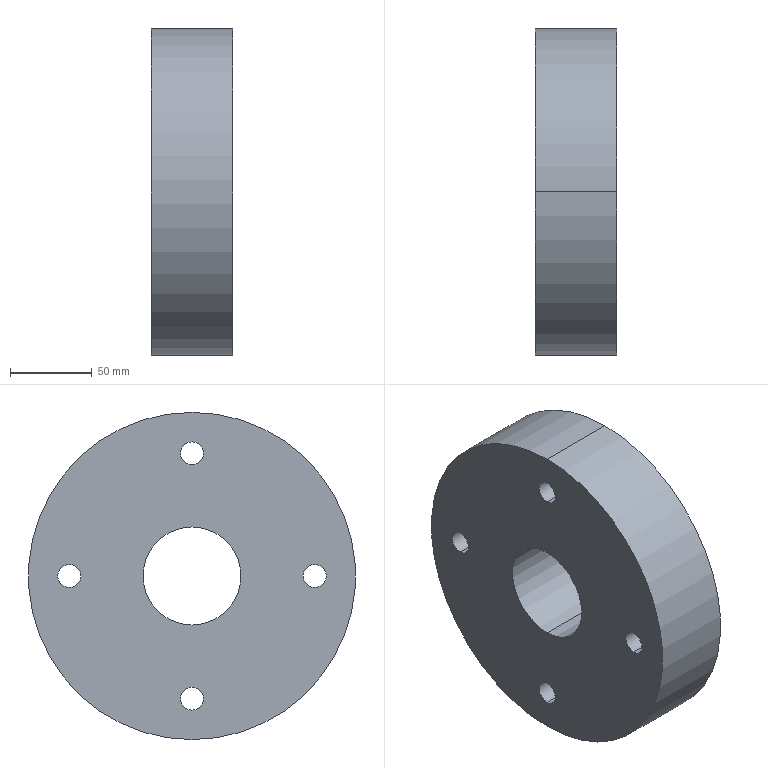Part | SolidWorks | features 3DProfileFeature 1, CirPattern 1, HoleWzd 1, Revolution 1 | 1 solid | 14 faces | box 50 x 200 x 200 mm | volume 1398637 mm3 | cylinder 12 | plane 2 | commonest cylinder face diameters 14 x8 60 x2 200 x2
STEP:
#1=CARTESIAN_POINT('',(25.,-75.,-7.));
#2=VERTEX_POINT('',#1);
#3=CARTESIAN_POINT('',(25.,-75.,7.));
#4=VERTEX_POINT('',#3);
#5=CARTESIAN_POINT('',(25.,-75.,0.));
#6=DIRECTION('',(-1.,0.,0.));
#7=DIRECTION('',(0.,0.,1.));
#8=AXIS2_PLACEMENT_3D('',#5,#6,#7);
#9=CIRCLE('',#8,7.);
#10=EDGE_CURVE('',#2,#4,#9,.T.);
#11=ORIENTED_EDGE('',*,*,#10,.F.);
#12=CARTESIAN_POINT('',(-25.,-75.,-7.));
#13=VERTEX_POINT('',#12);
#14=CARTESIAN_POINT('',(-25.,-75.,-7.));
#15=DIRECTION('',(-1.,0.,0.));
#16=VECTOR('',#15,1000.);
#17=LINE('',#14,#16);
#18=EDGE_CURVE('',#2,#13,#17,.T.);
#19=ORIENTED_EDGE('',*,*,#18,.T.);
#20=CARTESIAN_POINT('',(-25.,-75.,7.));
#21=VERTEX_POINT('',#20);
#22=CARTESIAN_POINT('',(-25.,-75.,0.));
#23=DIRECTION('',(-1.,0.,0.));
#24=DIRECTION('',(0.,0.,1.));
#25=AXIS2_PLACEMENT_3D('',#22,#23,#24);
#26=CIRCLE('',#25,7.);
#27=EDGE_CURVE('',#13,#21,#26,.T.);
#28=ORIENTED_EDGE('',*,*,#27,.T.);
#29=CARTESIAN_POINT('',(-25.,-75.,7.));
#30=DIRECTION('',(-1.,0.,0.));
#31=VECTOR('',#30,1000.);
#32=LINE('',#29,#31);
#33=EDGE_CURVE('',#4,#21,#32,.T.);
#34=ORIENTED_EDGE('',*,*,#33,.F.);
#35=EDGE_LOOP('',(#11,#19,#28,#34));
#36=FACE_OUTER_BOUND('',#35,.T.);
#37=CARTESIAN_POINT('',(-25.,-75.,0.));
#38=DIRECTION('',(-1.,0.,0.));
#39=DIRECTION('',(0.,0.,1.));
#40=AXIS2_PLACEMENT_3D('',#37,#38,#39);
#41=CYLINDRICAL_SURFACE('',#40,7.);
#42=ADVANCED_FACE('',(#36),#41,.F.);
#43=CARTESIAN_POINT('',(25.,0.,68.));
#44=VERTEX_POINT('',#43);
#45=CARTESIAN_POINT('',(25.,0.,82.));
#46=VERTEX_POINT('',#45);
#47=CARTESIAN_POINT('',(25.,0.,75.));
#48=DIRECTION('',(-1.,0.,0.));
#49=DIRECTION('',(0.,0.,1.));
#50=AXIS2_PLACEMENT_3D('',#47,#48,#49);
#51=CIRCLE('',#50,7.);
#52=EDGE_CURVE('',#44,#46,#51,.T.);
#53=ORIENTED_EDGE('',*,*,#52,.F.);
#54=CARTESIAN_POINT('',(-25.,0.,68.));
#55=VERTEX_POINT('',#54);
#56=CARTESIAN_POINT('',(-25.,0.,68.));
#57=DIRECTION('',(-1.,0.,0.));
#58=VECTOR('',#57,1000.);
#59=LINE('',#56,#58);
#60=EDGE_CURVE('',#44,#55,#59,.T.);
#61=ORIENTED_EDGE('',*,*,#60,.T.);
#62=CARTESIAN_POINT('',(-25.,0.,82.));
#63=VERTEX_POINT('',#62);
#64=CARTESIAN_POINT('',(-25.,0.,75.));
#65=DIRECTION('',(-1.,0.,0.));
#66=DIRECTION('',(0.,0.,1.));
#67=AXIS2_PLACEMENT_3D('',#64,#65,#66);
#68=CIRCLE('',#67,7.);
#69=EDGE_CURVE('',#55,#63,#68,.T.);
#70=ORIENTED_EDGE('',*,*,#69,.T.);
#71=CARTESIAN_POINT('',(-25.,0.,82.));
#72=DIRECTION('',(-1.,0.,0.));
#73=VECTOR('',#72,1000.);
#74=LINE('',#71,#73);
#75=EDGE_CURVE('',#46,#63,#74,.T.);
#76=ORIENTED_EDGE('',*,*,#75,.F.);
#77=EDGE_LOOP('',(#53,#61,#70,#76));
#78=FACE_OUTER_BOUND('',#77,.T.);
#79=CARTESIAN_POINT('',(-25.,0.,75.));
#80=DIRECTION('',(-1.,0.,0.));
#81=DIRECTION('',(0.,0.,1.));
#82=AXIS2_PLACEMENT_3D('',#79,#80,#81);
#83=CYLINDRICAL_SURFACE('',#82,7.);
#84=ADVANCED_FACE('',(#78),#83,.F.);
#85=CARTESIAN_POINT('',(25.,75.,-7.));
#86=VERTEX_POINT('',#85);
#87=CARTESIAN_POINT('',(25.,75.,7.));
#88=VERTEX_POINT('',#87);
#89=CARTESIAN_POINT('',(25.,75.,0.));
#90=DIRECTION('',(-1.,0.,0.));
#91=DIRECTION('',(0.,0.,1.));
#92=AXIS2_PLACEMENT_3D('',#89,#90,#91);
#93=CIRCLE('',#92,7.);
#94=EDGE_CURVE('',#86,#88,#93,.T.);
#95=ORIENTED_EDGE('',*,*,#94,.F.);
#96=CARTESIAN_POINT('',(-25.,75.,-7.));
#97=VERTEX_POINT('',#96);
#98=CARTESIAN_POINT('',(-25.,75.,-7.));
#99=DIRECTION('',(-1.,0.,0.));
#100=VECTOR('',#99,1000.);
#101=LINE('',#98,#100);
#102=EDGE_CURVE('',#86,#97,#101,.T.);
#103=ORIENTED_EDGE('',*,*,#102,.T.);
#104=CARTESIAN_POINT('',(-25.,75.,7.));
#105=VERTEX_POINT('',#104);
#106=CARTESIAN_POINT('',(-25.,75.,0.));
#107=DIRECTION('',(-1.,0.,0.));
#108=DIRECTION('',(0.,0.,1.));
#109=AXIS2_PLACEMENT_3D('',#106,#107,#108);
#110=CIRCLE('',#109,7.);
#111=EDGE_CURVE('',#97,#105,#110,.T.);
#112=ORIENTED_EDGE('',*,*,#111,.T.);
#113=CARTESIAN_POINT('',(-25.,75.,7.));
#114=DIRECTION('',(-1.,0.,0.));
#115=VECTOR('',#114,1000.);
#116=LINE('',#113,#115);
#117=EDGE_CURVE('',#88,#105,#116,.T.);
#118=ORIENTED_EDGE('',*,*,#117,.F.);
#119=EDGE_LOOP('',(#95,#103,#112,#118));
#120=FACE_OUTER_BOUND('',#119,.T.);
#121=CARTESIAN_POINT('',(-25.,75.,0.));
#122=DIRECTION('',(-1.,0.,0.));
#123=DIRECTION('',(0.,0.,1.));
#124=AXIS2_PLACEMENT_3D('',#121,#122,#123);
#125=CYLINDRICAL_SURFACE('',#124,7.);
#126=ADVANCED_FACE('',(#120),#125,.F.);
#127=CARTESIAN_POINT('',(25.,0.,-82.));
#128=VERTEX_POINT('',#127);
#129=CARTESIAN_POINT('',(25.,0.,-68.));
#130=VERTEX_POINT('',#129);
#131=CARTESIAN_POINT('',(25.,0.,-75.));
#132=DIRECTION('',(-1.,0.,0.));
#133=DIRECTION('',(0.,0.,1.));
#134=AXIS2_PLACEMENT_3D('',#131,#132,#133);
#135=CIRCLE('',#134,7.);
#136=EDGE_CURVE('',#128,#130,#135,.T.);
#137=ORIENTED_EDGE('',*,*,#136,.F.);
#138=CARTESIAN_POINT('',(-25.,0.,-82.));
#139=VERTEX_POINT('',#138);
#140=CARTESIAN_POINT('',(-25.,0.,-82.));
#141=DIRECTION('',(-1.,0.,0.));
#142=VECTOR('',#141,1000.);
#143=LINE('',#140,#142);
#144=EDGE_CURVE('',#128,#139,#143,.T.);
#145=ORIENTED_EDGE('',*,*,#144,.T.);
#146=CARTESIAN_POINT('',(-25.,0.,-68.));
#147=VERTEX_POINT('',#146);
#148=CARTESIAN_POINT('',(-25.,0.,-75.));
#149=DIRECTION('',(-1.,0.,0.));
#150=DIRECTION('',(0.,0.,1.));
#151=AXIS2_PLACEMENT_3D('',#148,#149,#150);
#152=CIRCLE('',#151,7.);
#153=EDGE_CURVE('',#139,#147,#152,.T.);
#154=ORIENTED_EDGE('',*,*,#153,.T.);
#155=CARTESIAN_POINT('',(-25.,0.,-68.));
#156=DIRECTION('',(-1.,0.,0.));
#157=VECTOR('',#156,1000.);
#158=LINE('',#155,#157);
#159=EDGE_CURVE('',#130,#147,#158,.T.);
#160=ORIENTED_EDGE('',*,*,#159,.F.);
#161=EDGE_LOOP('',(#137,#145,#154,#160));
#162=FACE_OUTER_BOUND('',#161,.T.);
#163=CARTESIAN_POINT('',(-25.,0.,-75.));
#164=DIRECTION('',(-1.,0.,0.));
#165=DIRECTION('',(0.,0.,1.));
#166=AXIS2_PLACEMENT_3D('',#163,#164,#165);
#167=CYLINDRICAL_SURFACE('',#166,7.);
#168=ADVANCED_FACE('',(#162),#167,.F.);
#169=CARTESIAN_POINT('',(-25.,0.,-100.));
#170=VERTEX_POINT('',#169);
#171=CARTESIAN_POINT('',(-25.,0.,100.));
#172=VERTEX_POINT('',#171);
#173=CARTESIAN_POINT('',(-25.,0.,0.));
#174=DIRECTION('',(1.,0.,0.));
#175=DIRECTION('',(0.,0.,-1.));
#176=AXIS2_PLACEMENT_3D('',#173,#174,#175);
#177=CIRCLE('',#176,100.);
#178=EDGE_CURVE('',#170,#172,#177,.T.);
#179=ORIENTED_EDGE('',*,*,#178,.T.);
#180=CARTESIAN_POINT('',(25.,0.,100.));
#181=VERTEX_POINT('',#180);
#182=CARTESIAN_POINT('',(71.901,0.,100.));
#183=DIRECTION('',(1.,0.,0.));
#184=VECTOR('',#183,1000.);
#185=LINE('',#182,#184);
#186=EDGE_CURVE('',#172,#181,#185,.T.);
#187=ORIENTED_EDGE('',*,*,#186,.T.);
#188=CARTESIAN_POINT('',(25.,0.,-100.));
#189=VERTEX_POINT('',#188);
#190=CARTESIAN_POINT('',(25.,0.,0.));
#191=DIRECTION('',(1.,0.,0.));
#192=DIRECTION('',(0.,0.,-1.));
#193=AXIS2_PLACEMENT_3D('',#190,#191,#192);
#194=CIRCLE('',#193,100.);
#195=EDGE_CURVE('',#189,#181,#194,.T.);
#196=ORIENTED_EDGE('',*,*,#195,.F.);
#197=CARTESIAN_POINT('',(71.901,0.,-100.));
#198=DIRECTION('',(1.,0.,0.));
#199=VECTOR('',#198,1000.);
#200=LINE('',#197,#199);
#201=EDGE_CURVE('',#170,#189,#200,.T.);
#202=ORIENTED_EDGE('',*,*,#201,.F.);
#203=EDGE_LOOP('',(#179,#187,#196,#202));
#204=FACE_OUTER_BOUND('',#203,.T.);
#205=CARTESIAN_POINT('',(71.901,0.,0.));
#206=DIRECTION('',(1.,0.,0.));
#207=DIRECTION('',(0.,0.,-1.));
#208=AXIS2_PLACEMENT_3D('',#205,#206,#207);
#209=CYLINDRICAL_SURFACE('',#208,100.);
#210=ADVANCED_FACE('',(#204),#209,.T.);
#211=CARTESIAN_POINT('',(-25.,0.,30.));
#212=VERTEX_POINT('',#211);
#213=CARTESIAN_POINT('',(-25.,0.,-30.));
#214=VERTEX_POINT('',#213);
#215=CARTESIAN_POINT('',(-25.,0.,0.));
#216=DIRECTION('',(1.,0.,0.));
#217=DIRECTION('',(0.,0.,-1.));
#218=AXIS2_PLACEMENT_3D('',#215,#216,#217);
#219=CIRCLE('',#218,30.);
#220=EDGE_CURVE('',#212,#214,#219,.T.);
#221=ORIENTED_EDGE('',*,*,#220,.F.);
#222=CARTESIAN_POINT('',(25.,0.,30.));
#223=VERTEX_POINT('',#222);
#224=CARTESIAN_POINT('',(71.901,0.,30.));
#225=DIRECTION('',(1.,0.,0.));
#226=VECTOR('',#225,1000.);
#227=LINE('',#224,#226);
#228=EDGE_CURVE('',#212,#223,#227,.T.);
#229=ORIENTED_EDGE('',*,*,#228,.T.);
#230=CARTESIAN_POINT('',(25.,0.,-30.));
#231=VERTEX_POINT('',#230);
#232=CARTESIAN_POINT('',(25.,0.,0.));
#233=DIRECTION('',(1.,0.,0.));
#234=DIRECTION('',(0.,0.,-1.));
#235=AXIS2_PLACEMENT_3D('',#232,#233,#234);
#236=CIRCLE('',#235,30.);
#237=EDGE_CURVE('',#223,#231,#236,.T.);
#238=ORIENTED_EDGE('',*,*,#237,.T.);
#239=CARTESIAN_POINT('',(71.901,0.,-30.));
#240=DIRECTION('',(1.,0.,0.));
#241=VECTOR('',#240,1000.);
#242=LINE('',#239,#241);
#243=EDGE_CURVE('',#214,#231,#242,.T.);
#244=ORIENTED_EDGE('',*,*,#243,.F.);
#245=EDGE_LOOP('',(#221,#229,#238,#244));
#246=FACE_OUTER_BOUND('',#245,.T.);
#247=CARTESIAN_POINT('',(71.901,0.,0.));
#248=DIRECTION('',(1.,0.,0.));
#249=DIRECTION('',(0.,0.,-1.));
#250=AXIS2_PLACEMENT_3D('',#247,#248,#249);
#251=CYLINDRICAL_SURFACE('',#250,30.);
#252=ADVANCED_FACE('',(#246),#251,.F.);
#253=CARTESIAN_POINT('',(25.,-75.,0.));
#254=DIRECTION('',(-1.,0.,0.));
#255=DIRECTION('',(0.,0.,1.));
#256=AXIS2_PLACEMENT_3D('',#253,#254,#255);
#257=CIRCLE('',#256,7.);
#258=EDGE_CURVE('',#4,#2,#257,.T.);
#259=ORIENTED_EDGE('',*,*,#258,.T.);
#260=ORIENTED_EDGE('',*,*,#10,.T.);
#261=EDGE_LOOP('',(#259,#260));
#262=FACE_BOUND('',#261,.T.);
#263=CARTESIAN_POINT('',(25.,0.,75.));
#264=DIRECTION('',(-1.,0.,0.));
#265=DIRECTION('',(0.,0.,1.));
#266=AXIS2_PLACEMENT_3D('',#263,#264,#265);
#267=CIRCLE('',#266,7.);
#268=EDGE_CURVE('',#46,#44,#267,.T.);
#269=ORIENTED_EDGE('',*,*,#268,.T.);
#270=ORIENTED_EDGE('',*,*,#52,.T.);
#271=EDGE_LOOP('',(#269,#270));
#272=FACE_BOUND('',#271,.T.);
#273=CARTESIAN_POINT('',(25.,75.,0.));
#274=DIRECTION('',(-1.,0.,0.));
#275=DIRECTION('',(0.,0.,1.));
#276=AXIS2_PLACEMENT_3D('',#273,#274,#275);
#277=CIRCLE('',#276,7.);
#278=EDGE_CURVE('',#88,#86,#277,.T.);
#279=ORIENTED_EDGE('',*,*,#278,.T.);
#280=ORIENTED_EDGE('',*,*,#94,.T.);
#281=EDGE_LOOP('',(#279,#280));
#282=FACE_BOUND('',#281,.T.);
#283=CARTESIAN_POINT('',(25.,0.,-75.));
#284=DIRECTION('',(-1.,0.,0.));
#285=DIRECTION('',(0.,0.,1.));
#286=AXIS2_PLACEMENT_3D('',#283,#284,#285);
#287=CIRCLE('',#286,7.);
#288=EDGE_CURVE('',#130,#128,#287,.T.);
#289=ORIENTED_EDGE('',*,*,#288,.T.);
#290=ORIENTED_EDGE('',*,*,#136,.T.);
#291=EDGE_LOOP('',(#289,#290));
#292=FACE_BOUND('',#291,.T.);
#293=ORIENTED_EDGE('',*,*,#195,.T.);
#294=CARTESIAN_POINT('',(25.,0.,0.));
#295=DIRECTION('',(1.,0.,0.));
#296=DIRECTION('',(0.,0.,-1.));
#297=AXIS2_PLACEMENT_3D('',#294,#295,#296);
#298=CIRCLE('',#297,100.);
#299=EDGE_CURVE('',#181,#189,#298,.T.);
#300=ORIENTED_EDGE('',*,*,#299,.T.);
#301=EDGE_LOOP('',(#293,#300));
#302=FACE_OUTER_BOUND('',#301,.T.);
#303=CARTESIAN_POINT('',(25.,0.,0.));
#304=DIRECTION('',(1.,0.,0.));
#305=DIRECTION('',(0.,0.,-1.));
#306=AXIS2_PLACEMENT_3D('',#303,#304,#305);
#307=CIRCLE('',#306,30.);
#308=EDGE_CURVE('',#231,#223,#307,.T.);
#309=ORIENTED_EDGE('',*,*,#308,.F.);
#310=ORIENTED_EDGE('',*,*,#237,.F.);
#311=EDGE_LOOP('',(#309,#310));
#312=FACE_BOUND('',#311,.T.);
#313=CARTESIAN_POINT('',(25.,30.,0.));
#314=DIRECTION('',(1.,0.,0.));
#315=DIRECTION('',(0.,0.,-1.));
#316=AXIS2_PLACEMENT_3D('',#313,#314,#315);
#317=PLANE('',#316);
#318=ADVANCED_FACE('',(#262,#272,#282,#292,#302,#312),#317,.T.);
#319=ORIENTED_EDGE('',*,*,#228,.F.);
#320=CARTESIAN_POINT('',(-25.,0.,0.));
#321=DIRECTION('',(1.,0.,0.));
#322=DIRECTION('',(0.,0.,-1.));
#323=AXIS2_PLACEMENT_3D('',#320,#321,#322);
#324=CIRCLE('',#323,30.);
#325=EDGE_CURVE('',#214,#212,#324,.T.);
#326=ORIENTED_EDGE('',*,*,#325,.F.);
#327=ORIENTED_EDGE('',*,*,#243,.T.);
#328=ORIENTED_EDGE('',*,*,#308,.T.);
#329=EDGE_LOOP('',(#319,#326,#327,#328));
#330=FACE_OUTER_BOUND('',#329,.T.);
#331=CARTESIAN_POINT('',(71.901,0.,0.));
#332=DIRECTION('',(1.,0.,0.));
#333=DIRECTION('',(0.,0.,-1.));
#334=AXIS2_PLACEMENT_3D('',#331,#332,#333);
#335=CYLINDRICAL_SURFACE('',#334,30.);
#336=ADVANCED_FACE('',(#330),#335,.F.);
#337=CARTESIAN_POINT('',(-25.,-75.,0.));
#338=DIRECTION('',(-1.,0.,0.));
#339=DIRECTION('',(0.,0.,1.));
#340=AXIS2_PLACEMENT_3D('',#337,#338,#339);
#341=CIRCLE('',#340,7.);
#342=EDGE_CURVE('',#21,#13,#341,.T.);
#343=ORIENTED_EDGE('',*,*,#342,.F.);
#344=ORIENTED_EDGE('',*,*,#27,.F.);
#345=EDGE_LOOP('',(#343,#344));
#346=FACE_BOUND('',#345,.T.);
#347=CARTESIAN_POINT('',(-25.,0.,75.));
#348=DIRECTION('',(-1.,0.,0.));
#349=DIRECTION('',(0.,0.,1.));
#350=AXIS2_PLACEMENT_3D('',#347,#348,#349);
#351=CIRCLE('',#350,7.);
#352=EDGE_CURVE('',#63,#55,#351,.T.);
#353=ORIENTED_EDGE('',*,*,#352,.F.);
#354=ORIENTED_EDGE('',*,*,#69,.F.);
#355=EDGE_LOOP('',(#353,#354));
#356=FACE_BOUND('',#355,.T.);
#357=CARTESIAN_POINT('',(-25.,75.,0.));
#358=DIRECTION('',(-1.,0.,0.));
#359=DIRECTION('',(0.,0.,1.));
#360=AXIS2_PLACEMENT_3D('',#357,#358,#359);
#361=CIRCLE('',#360,7.);
#362=EDGE_CURVE('',#105,#97,#361,.T.);
#363=ORIENTED_EDGE('',*,*,#362,.F.);
#364=ORIENTED_EDGE('',*,*,#111,.F.);
#365=EDGE_LOOP('',(#363,#364));
#366=FACE_BOUND('',#365,.T.);
#367=CARTESIAN_POINT('',(-25.,0.,-75.));
#368=DIRECTION('',(-1.,0.,0.));
#369=DIRECTION('',(0.,0.,1.));
#370=AXIS2_PLACEMENT_3D('',#367,#368,#369);
#371=CIRCLE('',#370,7.);
#372=EDGE_CURVE('',#147,#139,#371,.T.);
#373=ORIENTED_EDGE('',*,*,#372,.F.);
#374=ORIENTED_EDGE('',*,*,#153,.F.);
#375=EDGE_LOOP('',(#373,#374));
#376=FACE_BOUND('',#375,.T.);
#377=ORIENTED_EDGE('',*,*,#325,.T.);
#378=ORIENTED_EDGE('',*,*,#220,.T.);
#379=EDGE_LOOP('',(#377,#378));
#380=FACE_BOUND('',#379,.T.);
#381=ORIENTED_EDGE('',*,*,#178,.F.);
#382=CARTESIAN_POINT('',(-25.,0.,0.));
#383=DIRECTION('',(1.,0.,0.));
#384=DIRECTION('',(0.,0.,-1.));
#385=AXIS2_PLACEMENT_3D('',#382,#383,#384);
#386=CIRCLE('',#385,100.);
#387=EDGE_CURVE('',#172,#170,#386,.T.);
#388=ORIENTED_EDGE('',*,*,#387,.F.);
#389=EDGE_LOOP('',(#381,#388));
#390=FACE_OUTER_BOUND('',#389,.T.);
#391=CARTESIAN_POINT('',(-25.,30.,0.));
#392=DIRECTION('',(-1.,0.,0.));
#393=DIRECTION('',(0.,0.,1.));
#394=AXIS2_PLACEMENT_3D('',#391,#392,#393);
#395=PLANE('',#394);
#396=ADVANCED_FACE('',(#346,#356,#366,#376,#380,#390),#395,.T.);
#397=ORIENTED_EDGE('',*,*,#186,.F.);
#398=ORIENTED_EDGE('',*,*,#387,.T.);
#399=ORIENTED_EDGE('',*,*,#201,.T.);
#400=ORIENTED_EDGE('',*,*,#299,.F.);
#401=EDGE_LOOP('',(#397,#398,#399,#400));
#402=FACE_OUTER_BOUND('',#401,.T.);
#403=CARTESIAN_POINT('',(71.901,0.,0.));
#404=DIRECTION('',(1.,0.,0.));
#405=DIRECTION('',(0.,0.,-1.));
#406=AXIS2_PLACEMENT_3D('',#403,#404,#405);
#407=CYLINDRICAL_SURFACE('',#406,100.);
#408=ADVANCED_FACE('',(#402),#407,.T.);
#409=ORIENTED_EDGE('',*,*,#144,.F.);
#410=ORIENTED_EDGE('',*,*,#288,.F.);
#411=ORIENTED_EDGE('',*,*,#159,.T.);
#412=ORIENTED_EDGE('',*,*,#372,.T.);
#413=EDGE_LOOP('',(#409,#410,#411,#412));
#414=FACE_OUTER_BOUND('',#413,.T.);
#415=CARTESIAN_POINT('',(-25.,0.,-75.));
#416=DIRECTION('',(-1.,0.,0.));
#417=DIRECTION('',(0.,0.,1.));
#418=AXIS2_PLACEMENT_3D('',#415,#416,#417);
#419=CYLINDRICAL_SURFACE('',#418,7.);
#420=ADVANCED_FACE('',(#414),#419,.F.);
#421=ORIENTED_EDGE('',*,*,#102,.F.);
#422=ORIENTED_EDGE('',*,*,#278,.F.);
#423=ORIENTED_EDGE('',*,*,#117,.T.);
#424=ORIENTED_EDGE('',*,*,#362,.T.);
#425=EDGE_LOOP('',(#421,#422,#423,#424));
#426=FACE_OUTER_BOUND('',#425,.T.);
#427=CARTESIAN_POINT('',(-25.,75.,0.));
#428=DIRECTION('',(-1.,0.,0.));
#429=DIRECTION('',(0.,0.,1.));
#430=AXIS2_PLACEMENT_3D('',#427,#428,#429);
#431=CYLINDRICAL_SURFACE('',#430,7.);
#432=ADVANCED_FACE('',(#426),#431,.F.);
#433=ORIENTED_EDGE('',*,*,#60,.F.);
#434=ORIENTED_EDGE('',*,*,#268,.F.);
#435=ORIENTED_EDGE('',*,*,#75,.T.);
#436=ORIENTED_EDGE('',*,*,#352,.T.);
#437=EDGE_LOOP('',(#433,#434,#435,#436));
#438=FACE_OUTER_BOUND('',#437,.T.);
#439=CARTESIAN_POINT('',(-25.,0.,75.));
#440=DIRECTION('',(-1.,0.,0.));
#441=DIRECTION('',(0.,0.,1.));
#442=AXIS2_PLACEMENT_3D('',#439,#440,#441);
#443=CYLINDRICAL_SURFACE('',#442,7.);
#444=ADVANCED_FACE('',(#438),#443,.F.);
#445=ORIENTED_EDGE('',*,*,#18,.F.);
#446=ORIENTED_EDGE('',*,*,#258,.F.);
#447=ORIENTED_EDGE('',*,*,#33,.T.);
#448=ORIENTED_EDGE('',*,*,#342,.T.);
#449=EDGE_LOOP('',(#445,#446,#447,#448));
#450=FACE_OUTER_BOUND('',#449,.T.);
#451=CARTESIAN_POINT('',(-25.,-75.,0.));
#452=DIRECTION('',(-1.,0.,0.));
#453=DIRECTION('',(0.,0.,1.));
#454=AXIS2_PLACEMENT_3D('',#451,#452,#453);
#455=CYLINDRICAL_SURFACE('',#454,7.);
#456=ADVANCED_FACE('',(#450),#455,.F.);
#457=CLOSED_SHELL('',(#42,#84,#126,#168,#210,#252,#318,#336,#396,#408,#420,#432,#444,#456));
#458=MANIFOLD_SOLID_BREP('',#457);
#459=CARTESIAN_POINT('',(0.,0.,0.));
#460=DIRECTION('',(0.,0.,1.));
#461=DIRECTION('',(1.,0.,0.));
#462=AXIS2_PLACEMENT_3D('',#459,#460,#461);
#463=(LENGTH_UNIT()NAMED_UNIT(*)SI_UNIT(.MILLI.,.METRE.));
#464=UNCERTAINTY_MEASURE_WITH_UNIT(LENGTH_MEASURE(0.00001),#463,'','');
#465=(NAMED_UNIT(*)PLANE_ANGLE_UNIT()SI_UNIT($,.RADIAN.));
#466=(NAMED_UNIT(*)SI_UNIT($,.STERADIAN.)SOLID_ANGLE_UNIT());
#467=(GEOMETRIC_REPRESENTATION_CONTEXT(3)GLOBAL_UNCERTAINTY_ASSIGNED_CONTEXT((#464))GLOBAL_UNIT_ASSIGNED_CONTEXT((#463,#465,#466))REPRESENTATION_CONTEXT('',''));
#468=ADVANCED_BREP_SHAPE_REPRESENTATION('',(#458,#462),#467);